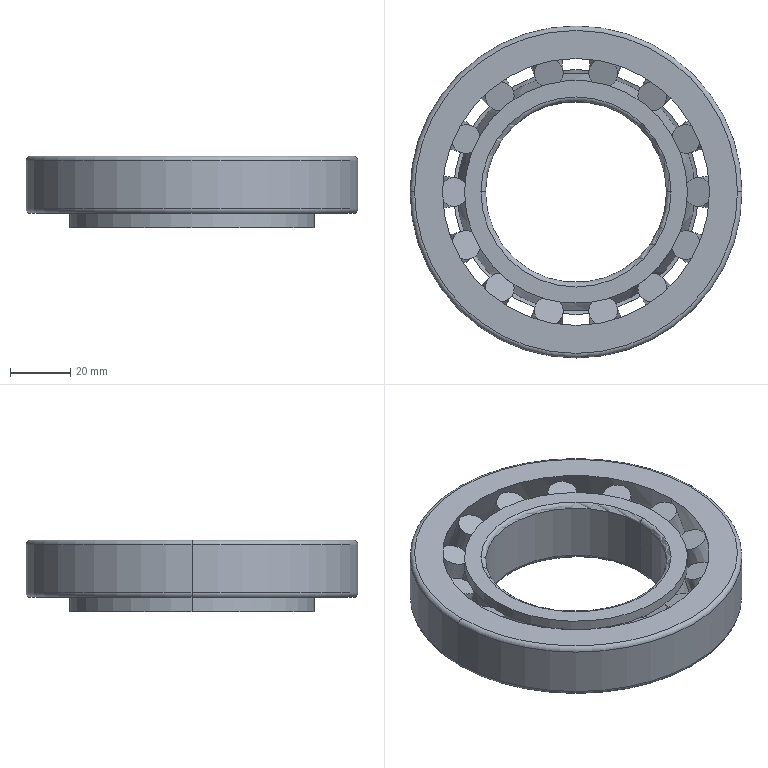Part | SolidWorks | features Revolution 3, CirPattern 1, RefAxis 1 | 16 solids | 84 faces | box 110 x 110 x 23.75 mm | volume 99451 mm3 | cone 36 | plane 32 | cylinder 8 | torus 8 | commonest cylinder face diameters 60 x2 73.881 x2 81.198 x2 110 x2